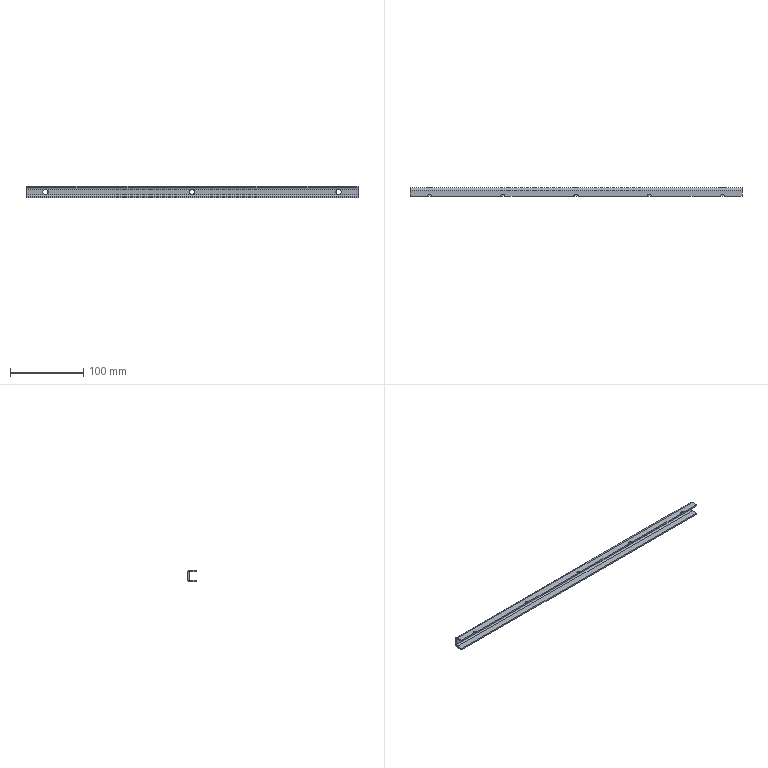Part | NX | features solid 2 | 1 solid | 35 faces | box 453 x 12 x 16 mm | volume 29904 mm3 | cylinder 20 | plane 15 | commonest cylinder face diameters 6 x10 7.1 x6 4 x2 8 x2
STEP:
#1=CARTESIAN_POINT('',(1406.5,-1575.5,344.5));
#2=VERTEX_POINT('',#1);
#3=CARTESIAN_POINT('',(1406.5,-1575.5,346.5));
#4=VERTEX_POINT('',#3);
#5=CARTESIAN_POINT('',(1406.5,-1575.5,346.5));
#6=DIRECTION('',(0.,0.,1.));
#7=VECTOR('',#6,1000.);
#8=LINE('',#5,#7);
#9=EDGE_CURVE('',#2,#4,#8,.T.);
#10=ORIENTED_EDGE('',*,*,#9,.F.);
#11=CARTESIAN_POINT('',(1409.5,-1578.5,344.5));
#12=VERTEX_POINT('',#11);
#13=CARTESIAN_POINT('',(1406.5,-1578.5,344.5));
#14=DIRECTION('',(0.,0.,-1.));
#15=DIRECTION('',(0.,1.,0.));
#16=AXIS2_PLACEMENT_3D('',#13,#14,#15);
#17=CIRCLE('',#16,3.);
#18=EDGE_CURVE('',#2,#12,#17,.T.);
#19=ORIENTED_EDGE('',*,*,#18,.T.);
#20=CARTESIAN_POINT('',(1409.5,-1578.5,346.5));
#21=VERTEX_POINT('',#20);
#22=CARTESIAN_POINT('',(1409.5,-1578.5,346.5));
#23=DIRECTION('',(0.,0.,1.));
#24=VECTOR('',#23,1000.);
#25=LINE('',#22,#24);
#26=EDGE_CURVE('',#12,#21,#25,.T.);
#27=ORIENTED_EDGE('',*,*,#26,.T.);
#28=CARTESIAN_POINT('',(1406.5,-1578.5,346.5));
#29=DIRECTION('',(0.,0.,-1.));
#30=DIRECTION('',(0.,1.,0.));
#31=AXIS2_PLACEMENT_3D('',#28,#29,#30);
#32=CIRCLE('',#31,3.);
#33=EDGE_CURVE('',#4,#21,#32,.T.);
#34=ORIENTED_EDGE('',*,*,#33,.F.);
#35=EDGE_LOOP('',(#10,#19,#27,#34));
#36=FACE_BOUND('',#35,.T.);
#37=CARTESIAN_POINT('',(1406.5,-1578.5,346.5));
#38=DIRECTION('',(0.,0.,1.));
#39=DIRECTION('',(0.,1.,0.));
#40=AXIS2_PLACEMENT_3D('',#37,#38,#39);
#41=CYLINDRICAL_SURFACE('',#40,3.);
#42=ADVANCED_FACE('',(#36),#41,.F.);
#43=CARTESIAN_POINT('',(1506.5,-1575.5,344.5));
#44=VERTEX_POINT('',#43);
#45=CARTESIAN_POINT('',(1506.5,-1575.5,346.5));
#46=VERTEX_POINT('',#45);
#47=CARTESIAN_POINT('',(1506.5,-1575.5,346.5));
#48=DIRECTION('',(0.,0.,1.));
#49=VECTOR('',#48,1000.);
#50=LINE('',#47,#49);
#51=EDGE_CURVE('',#44,#46,#50,.T.);
#52=ORIENTED_EDGE('',*,*,#51,.F.);
#53=CARTESIAN_POINT('',(1509.5,-1578.5,344.5));
#54=VERTEX_POINT('',#53);
#55=CARTESIAN_POINT('',(1506.5,-1578.5,344.5));
#56=DIRECTION('',(0.,0.,-1.));
#57=DIRECTION('',(0.,1.,0.));
#58=AXIS2_PLACEMENT_3D('',#55,#56,#57);
#59=CIRCLE('',#58,3.);
#60=EDGE_CURVE('',#44,#54,#59,.T.);
#61=ORIENTED_EDGE('',*,*,#60,.T.);
#62=CARTESIAN_POINT('',(1509.5,-1578.5,346.5));
#63=VERTEX_POINT('',#62);
#64=CARTESIAN_POINT('',(1509.5,-1578.5,346.5));
#65=DIRECTION('',(0.,0.,1.));
#66=VECTOR('',#65,1000.);
#67=LINE('',#64,#66);
#68=EDGE_CURVE('',#54,#63,#67,.T.);
#69=ORIENTED_EDGE('',*,*,#68,.T.);
#70=CARTESIAN_POINT('',(1506.5,-1578.5,346.5));
#71=DIRECTION('',(0.,0.,-1.));
#72=DIRECTION('',(0.,1.,0.));
#73=AXIS2_PLACEMENT_3D('',#70,#71,#72);
#74=CIRCLE('',#73,3.);
#75=EDGE_CURVE('',#46,#63,#74,.T.);
#76=ORIENTED_EDGE('',*,*,#75,.F.);
#77=EDGE_LOOP('',(#52,#61,#69,#76));
#78=FACE_BOUND('',#77,.T.);
#79=CARTESIAN_POINT('',(1506.5,-1578.5,346.5));
#80=DIRECTION('',(0.,0.,1.));
#81=DIRECTION('',(0.,1.,0.));
#82=AXIS2_PLACEMENT_3D('',#79,#80,#81);
#83=CYLINDRICAL_SURFACE('',#82,3.);
#84=ADVANCED_FACE('',(#78),#83,.F.);
#85=CARTESIAN_POINT('',(1806.5,-1575.5,344.5));
#86=VERTEX_POINT('',#85);
#87=CARTESIAN_POINT('',(1806.5,-1575.5,346.5));
#88=VERTEX_POINT('',#87);
#89=CARTESIAN_POINT('',(1806.5,-1575.5,346.5));
#90=DIRECTION('',(0.,0.,1.));
#91=VECTOR('',#90,1000.);
#92=LINE('',#89,#91);
#93=EDGE_CURVE('',#86,#88,#92,.T.);
#94=ORIENTED_EDGE('',*,*,#93,.F.);
#95=CARTESIAN_POINT('',(1809.5,-1578.5,344.5));
#96=VERTEX_POINT('',#95);
#97=CARTESIAN_POINT('',(1806.5,-1578.5,344.5));
#98=DIRECTION('',(0.,0.,-1.));
#99=DIRECTION('',(0.,1.,0.));
#100=AXIS2_PLACEMENT_3D('',#97,#98,#99);
#101=CIRCLE('',#100,3.);
#102=EDGE_CURVE('',#86,#96,#101,.T.);
#103=ORIENTED_EDGE('',*,*,#102,.T.);
#104=CARTESIAN_POINT('',(1809.5,-1578.5,346.5));
#105=VERTEX_POINT('',#104);
#106=CARTESIAN_POINT('',(1809.5,-1578.5,346.5));
#107=DIRECTION('',(0.,0.,1.));
#108=VECTOR('',#107,1000.);
#109=LINE('',#106,#108);
#110=EDGE_CURVE('',#96,#105,#109,.T.);
#111=ORIENTED_EDGE('',*,*,#110,.T.);
#112=CARTESIAN_POINT('',(1806.5,-1578.5,346.5));
#113=DIRECTION('',(0.,0.,-1.));
#114=DIRECTION('',(0.,1.,0.));
#115=AXIS2_PLACEMENT_3D('',#112,#113,#114);
#116=CIRCLE('',#115,3.);
#117=EDGE_CURVE('',#88,#105,#116,.T.);
#118=ORIENTED_EDGE('',*,*,#117,.F.);
#119=EDGE_LOOP('',(#94,#103,#111,#118));
#120=FACE_BOUND('',#119,.T.);
#121=CARTESIAN_POINT('',(1806.5,-1578.5,346.5));
#122=DIRECTION('',(0.,0.,1.));
#123=DIRECTION('',(0.,1.,0.));
#124=AXIS2_PLACEMENT_3D('',#121,#122,#123);
#125=CYLINDRICAL_SURFACE('',#124,3.);
#126=ADVANCED_FACE('',(#120),#125,.F.);
#127=CARTESIAN_POINT('',(1706.5,-1575.5,344.5));
#128=VERTEX_POINT('',#127);
#129=CARTESIAN_POINT('',(1706.5,-1575.5,346.5));
#130=VERTEX_POINT('',#129);
#131=CARTESIAN_POINT('',(1706.5,-1575.5,346.5));
#132=DIRECTION('',(0.,0.,1.));
#133=VECTOR('',#132,1000.);
#134=LINE('',#131,#133);
#135=EDGE_CURVE('',#128,#130,#134,.T.);
#136=ORIENTED_EDGE('',*,*,#135,.F.);
#137=CARTESIAN_POINT('',(1709.5,-1578.5,344.5));
#138=VERTEX_POINT('',#137);
#139=CARTESIAN_POINT('',(1706.5,-1578.5,344.5));
#140=DIRECTION('',(0.,0.,-1.));
#141=DIRECTION('',(0.,1.,0.));
#142=AXIS2_PLACEMENT_3D('',#139,#140,#141);
#143=CIRCLE('',#142,3.);
#144=EDGE_CURVE('',#128,#138,#143,.T.);
#145=ORIENTED_EDGE('',*,*,#144,.T.);
#146=CARTESIAN_POINT('',(1709.5,-1578.5,346.5));
#147=VERTEX_POINT('',#146);
#148=CARTESIAN_POINT('',(1709.5,-1578.5,346.5));
#149=DIRECTION('',(0.,0.,1.));
#150=VECTOR('',#149,1000.);
#151=LINE('',#148,#150);
#152=EDGE_CURVE('',#138,#147,#151,.T.);
#153=ORIENTED_EDGE('',*,*,#152,.T.);
#154=CARTESIAN_POINT('',(1706.5,-1578.5,346.5));
#155=DIRECTION('',(0.,0.,-1.));
#156=DIRECTION('',(0.,1.,0.));
#157=AXIS2_PLACEMENT_3D('',#154,#155,#156);
#158=CIRCLE('',#157,3.);
#159=EDGE_CURVE('',#130,#147,#158,.T.);
#160=ORIENTED_EDGE('',*,*,#159,.F.);
#161=EDGE_LOOP('',(#136,#145,#153,#160));
#162=FACE_BOUND('',#161,.T.);
#163=CARTESIAN_POINT('',(1706.5,-1578.5,346.5));
#164=DIRECTION('',(0.,0.,1.));
#165=DIRECTION('',(0.,1.,0.));
#166=AXIS2_PLACEMENT_3D('',#163,#164,#165);
#167=CYLINDRICAL_SURFACE('',#166,3.);
#168=ADVANCED_FACE('',(#162),#167,.F.);
#169=CARTESIAN_POINT('',(1606.5,-1575.5,344.5));
#170=VERTEX_POINT('',#169);
#171=CARTESIAN_POINT('',(1606.5,-1575.5,346.5));
#172=VERTEX_POINT('',#171);
#173=CARTESIAN_POINT('',(1606.5,-1575.5,346.5));
#174=DIRECTION('',(0.,0.,1.));
#175=VECTOR('',#174,1000.);
#176=LINE('',#173,#175);
#177=EDGE_CURVE('',#170,#172,#176,.T.);
#178=ORIENTED_EDGE('',*,*,#177,.F.);
#179=CARTESIAN_POINT('',(1609.5,-1578.5,344.5));
#180=VERTEX_POINT('',#179);
#181=CARTESIAN_POINT('',(1606.5,-1578.5,344.5));
#182=DIRECTION('',(0.,0.,-1.));
#183=DIRECTION('',(0.,1.,0.));
#184=AXIS2_PLACEMENT_3D('',#181,#182,#183);
#185=CIRCLE('',#184,3.);
#186=EDGE_CURVE('',#170,#180,#185,.T.);
#187=ORIENTED_EDGE('',*,*,#186,.T.);
#188=CARTESIAN_POINT('',(1609.5,-1578.5,346.5));
#189=VERTEX_POINT('',#188);
#190=CARTESIAN_POINT('',(1609.5,-1578.5,346.5));
#191=DIRECTION('',(0.,0.,1.));
#192=VECTOR('',#191,1000.);
#193=LINE('',#190,#192);
#194=EDGE_CURVE('',#180,#189,#193,.T.);
#195=ORIENTED_EDGE('',*,*,#194,.T.);
#196=CARTESIAN_POINT('',(1606.5,-1578.5,346.5));
#197=DIRECTION('',(0.,0.,-1.));
#198=DIRECTION('',(0.,1.,0.));
#199=AXIS2_PLACEMENT_3D('',#196,#197,#198);
#200=CIRCLE('',#199,3.);
#201=EDGE_CURVE('',#172,#189,#200,.T.);
#202=ORIENTED_EDGE('',*,*,#201,.F.);
#203=EDGE_LOOP('',(#178,#187,#195,#202));
#204=FACE_BOUND('',#203,.T.);
#205=CARTESIAN_POINT('',(1606.5,-1578.5,346.5));
#206=DIRECTION('',(0.,0.,1.));
#207=DIRECTION('',(0.,1.,0.));
#208=AXIS2_PLACEMENT_3D('',#205,#206,#207);
#209=CYLINDRICAL_SURFACE('',#208,3.);
#210=ADVANCED_FACE('',(#204),#209,.F.);
#211=CARTESIAN_POINT('',(1380.,-1568.5,342.5));
#212=VERTEX_POINT('',#211);
#213=CARTESIAN_POINT('',(1833.,-1568.5,342.5));
#214=VERTEX_POINT('',#213);
#215=CARTESIAN_POINT('',(1380.,-1568.5,342.5));
#216=DIRECTION('',(1.,0.,0.));
#217=VECTOR('',#216,1000.);
#218=LINE('',#215,#217);
#219=EDGE_CURVE('',#212,#214,#218,.T.);
#220=ORIENTED_EDGE('',*,*,#219,.T.);
#221=CARTESIAN_POINT('',(1833.,-1570.5,344.5));
#222=VERTEX_POINT('',#221);
#223=CARTESIAN_POINT('',(1833.,-1570.5,342.5));
#224=DIRECTION('',(-1.,0.,0.));
#225=DIRECTION('',(0.,0.,1.));
#226=AXIS2_PLACEMENT_3D('',#223,#224,#225);
#227=CIRCLE('',#226,2.);
#228=EDGE_CURVE('',#222,#214,#227,.T.);
#229=ORIENTED_EDGE('',*,*,#228,.F.);
#230=CARTESIAN_POINT('',(1380.,-1570.5,344.5));
#231=VERTEX_POINT('',#230);
#232=CARTESIAN_POINT('',(1833.,-1570.5,344.5));
#233=DIRECTION('',(-1.,0.,0.));
#234=VECTOR('',#233,1000.);
#235=LINE('',#232,#234);
#236=EDGE_CURVE('',#222,#231,#235,.T.);
#237=ORIENTED_EDGE('',*,*,#236,.T.);
#238=CARTESIAN_POINT('',(1380.,-1570.5,342.5));
#239=DIRECTION('',(1.,0.,0.));
#240=DIRECTION('',(0.,0.,1.));
#241=AXIS2_PLACEMENT_3D('',#238,#239,#240);
#242=CIRCLE('',#241,2.);
#243=EDGE_CURVE('',#212,#231,#242,.T.);
#244=ORIENTED_EDGE('',*,*,#243,.F.);
#245=EDGE_LOOP('',(#220,#229,#237,#244));
#246=FACE_BOUND('',#245,.T.);
#247=CARTESIAN_POINT('',(1380.,-1570.5,342.5));
#248=DIRECTION('',(1.,0.,0.));
#249=DIRECTION('',(0.,-1.,0.));
#250=AXIS2_PLACEMENT_3D('',#247,#248,#249);
#251=CYLINDRICAL_SURFACE('',#250,2.);
#252=ADVANCED_FACE('',(#246),#251,.F.);
#253=CARTESIAN_POINT('',(1380.,-1566.5,342.5));
#254=VERTEX_POINT('',#253);
#255=CARTESIAN_POINT('',(1833.,-1566.5,342.5));
#256=VERTEX_POINT('',#255);
#257=CARTESIAN_POINT('',(1380.,-1566.5,342.5));
#258=DIRECTION('',(1.,0.,0.));
#259=VECTOR('',#258,1000.);
#260=LINE('',#257,#259);
#261=EDGE_CURVE('',#254,#256,#260,.T.);
#262=ORIENTED_EDGE('',*,*,#261,.F.);
#263=CARTESIAN_POINT('',(1380.,-1570.5,346.5));
#264=VERTEX_POINT('',#263);
#265=CARTESIAN_POINT('',(1380.,-1570.5,342.5));
#266=DIRECTION('',(1.,0.,0.));
#267=DIRECTION('',(0.,-1.,0.));
#268=AXIS2_PLACEMENT_3D('',#265,#266,#267);
#269=CIRCLE('',#268,4.);
#270=EDGE_CURVE('',#254,#264,#269,.T.);
#271=ORIENTED_EDGE('',*,*,#270,.T.);
#272=CARTESIAN_POINT('',(1833.,-1570.5,346.5));
#273=VERTEX_POINT('',#272);
#274=CARTESIAN_POINT('',(1833.,-1570.5,346.5));
#275=DIRECTION('',(-1.,0.,0.));
#276=VECTOR('',#275,1000.);
#277=LINE('',#274,#276);
#278=EDGE_CURVE('',#273,#264,#277,.T.);
#279=ORIENTED_EDGE('',*,*,#278,.F.);
#280=CARTESIAN_POINT('',(1833.,-1570.5,342.5));
#281=DIRECTION('',(-1.,0.,0.));
#282=DIRECTION('',(0.,-1.,0.));
#283=AXIS2_PLACEMENT_3D('',#280,#281,#282);
#284=CIRCLE('',#283,4.);
#285=EDGE_CURVE('',#273,#256,#284,.T.);
#286=ORIENTED_EDGE('',*,*,#285,.T.);
#287=EDGE_LOOP('',(#262,#271,#279,#286));
#288=FACE_BOUND('',#287,.T.);
#289=CARTESIAN_POINT('',(1380.,-1570.5,342.5));
#290=DIRECTION('',(1.,0.,0.));
#291=DIRECTION('',(0.,-1.,0.));
#292=AXIS2_PLACEMENT_3D('',#289,#290,#291);
#293=CYLINDRICAL_SURFACE('',#292,4.);
#294=ADVANCED_FACE('',(#288),#293,.T.);
#295=CARTESIAN_POINT('',(1833.,-1578.5,346.5));
#296=VERTEX_POINT('',#295);
#297=CARTESIAN_POINT('',(1380.,-1578.5,346.5));
#298=DIRECTION('',(1.,0.,0.));
#299=VECTOR('',#298,1000.);
#300=LINE('',#297,#299);
#301=EDGE_CURVE('',#105,#296,#300,.T.);
#302=ORIENTED_EDGE('',*,*,#301,.F.);
#303=ORIENTED_EDGE('',*,*,#110,.F.);
#304=CARTESIAN_POINT('',(1833.,-1578.5,344.5));
#305=VERTEX_POINT('',#304);
#306=CARTESIAN_POINT('',(1380.,-1578.5,344.5));
#307=DIRECTION('',(1.,0.,0.));
#308=VECTOR('',#307,1000.);
#309=LINE('',#306,#308);
#310=EDGE_CURVE('',#96,#305,#309,.T.);
#311=ORIENTED_EDGE('',*,*,#310,.T.);
#312=CARTESIAN_POINT('',(1833.,-1578.5,346.5));
#313=DIRECTION('',(0.,0.,-1.));
#314=VECTOR('',#313,1000.);
#315=LINE('',#312,#314);
#316=EDGE_CURVE('',#296,#305,#315,.T.);
#317=ORIENTED_EDGE('',*,*,#316,.F.);
#318=EDGE_LOOP('',(#302,#303,#311,#317));
#319=FACE_BOUND('',#318,.T.);
#320=CARTESIAN_POINT('',(1380.,-1578.5,346.5));
#321=DIRECTION('',(0.,1.,0.));
#322=DIRECTION('',(0.,0.,-1.));
#323=AXIS2_PLACEMENT_3D('',#320,#321,#322);
#324=PLANE('',#323);
#325=ADVANCED_FACE('',(#319),#324,.F.);
#326=CARTESIAN_POINT('',(1503.5,-1578.5,344.5));
#327=VERTEX_POINT('',#326);
#328=CARTESIAN_POINT('',(1380.,-1578.5,344.5));
#329=DIRECTION('',(1.,0.,0.));
#330=VECTOR('',#329,1000.);
#331=LINE('',#328,#330);
#332=EDGE_CURVE('',#12,#327,#331,.T.);
#333=ORIENTED_EDGE('',*,*,#332,.F.);
#334=ORIENTED_EDGE('',*,*,#18,.F.);
#335=CARTESIAN_POINT('',(1403.5,-1578.5,344.5));
#336=VERTEX_POINT('',#335);
#337=CARTESIAN_POINT('',(1406.5,-1578.5,344.5));
#338=DIRECTION('',(0.,0.,-1.));
#339=DIRECTION('',(0.,1.,0.));
#340=AXIS2_PLACEMENT_3D('',#337,#338,#339);
#341=CIRCLE('',#340,3.);
#342=EDGE_CURVE('',#336,#2,#341,.T.);
#343=ORIENTED_EDGE('',*,*,#342,.F.);
#344=CARTESIAN_POINT('',(1380.,-1578.5,344.5));
#345=VERTEX_POINT('',#344);
#346=CARTESIAN_POINT('',(1380.,-1578.5,344.5));
#347=DIRECTION('',(1.,0.,0.));
#348=VECTOR('',#347,1000.);
#349=LINE('',#346,#348);
#350=EDGE_CURVE('',#345,#336,#349,.T.);
#351=ORIENTED_EDGE('',*,*,#350,.F.);
#352=CARTESIAN_POINT('',(1380.,-1568.144,344.5));
#353=DIRECTION('',(0.,-1.,0.));
#354=VECTOR('',#353,1000.);
#355=LINE('',#352,#354);
#356=EDGE_CURVE('',#231,#345,#355,.T.);
#357=ORIENTED_EDGE('',*,*,#356,.F.);
#358=ORIENTED_EDGE('',*,*,#236,.F.);
#359=CARTESIAN_POINT('',(1833.,-1568.144,344.5));
#360=DIRECTION('',(0.,1.,0.));
#361=VECTOR('',#360,1000.);
#362=LINE('',#359,#361);
#363=EDGE_CURVE('',#305,#222,#362,.T.);
#364=ORIENTED_EDGE('',*,*,#363,.F.);
#365=ORIENTED_EDGE('',*,*,#310,.F.);
#366=ORIENTED_EDGE('',*,*,#102,.F.);
#367=CARTESIAN_POINT('',(1803.5,-1578.5,344.5));
#368=VERTEX_POINT('',#367);
#369=CARTESIAN_POINT('',(1806.5,-1578.5,344.5));
#370=DIRECTION('',(0.,0.,-1.));
#371=DIRECTION('',(0.,1.,0.));
#372=AXIS2_PLACEMENT_3D('',#369,#370,#371);
#373=CIRCLE('',#372,3.);
#374=EDGE_CURVE('',#368,#86,#373,.T.);
#375=ORIENTED_EDGE('',*,*,#374,.F.);
#376=CARTESIAN_POINT('',(1380.,-1578.5,344.5));
#377=DIRECTION('',(1.,0.,0.));
#378=VECTOR('',#377,1000.);
#379=LINE('',#376,#378);
#380=EDGE_CURVE('',#138,#368,#379,.T.);
#381=ORIENTED_EDGE('',*,*,#380,.F.);
#382=ORIENTED_EDGE('',*,*,#144,.F.);
#383=CARTESIAN_POINT('',(1703.5,-1578.5,344.5));
#384=VERTEX_POINT('',#383);
#385=CARTESIAN_POINT('',(1706.5,-1578.5,344.5));
#386=DIRECTION('',(0.,0.,-1.));
#387=DIRECTION('',(0.,1.,0.));
#388=AXIS2_PLACEMENT_3D('',#385,#386,#387);
#389=CIRCLE('',#388,3.);
#390=EDGE_CURVE('',#384,#128,#389,.T.);
#391=ORIENTED_EDGE('',*,*,#390,.F.);
#392=CARTESIAN_POINT('',(1380.,-1578.5,344.5));
#393=DIRECTION('',(1.,0.,0.));
#394=VECTOR('',#393,1000.);
#395=LINE('',#392,#394);
#396=EDGE_CURVE('',#180,#384,#395,.T.);
#397=ORIENTED_EDGE('',*,*,#396,.F.);
#398=ORIENTED_EDGE('',*,*,#186,.F.);
#399=CARTESIAN_POINT('',(1603.5,-1578.5,344.5));
#400=VERTEX_POINT('',#399);
#401=CARTESIAN_POINT('',(1606.5,-1578.5,344.5));
#402=DIRECTION('',(0.,0.,-1.));
#403=DIRECTION('',(0.,1.,0.));
#404=AXIS2_PLACEMENT_3D('',#401,#402,#403);
#405=CIRCLE('',#404,3.);
#406=EDGE_CURVE('',#400,#170,#405,.T.);
#407=ORIENTED_EDGE('',*,*,#406,.F.);
#408=CARTESIAN_POINT('',(1380.,-1578.5,344.5));
#409=DIRECTION('',(1.,0.,0.));
#410=VECTOR('',#409,1000.);
#411=LINE('',#408,#410);
#412=EDGE_CURVE('',#54,#400,#411,.T.);
#413=ORIENTED_EDGE('',*,*,#412,.F.);
#414=ORIENTED_EDGE('',*,*,#60,.F.);
#415=CARTESIAN_POINT('',(1506.5,-1578.5,344.5));
#416=DIRECTION('',(0.,0.,-1.));
#417=DIRECTION('',(0.,1.,0.));
#418=AXIS2_PLACEMENT_3D('',#415,#416,#417);
#419=CIRCLE('',#418,3.);
#420=EDGE_CURVE('',#327,#44,#419,.T.);
#421=ORIENTED_EDGE('',*,*,#420,.F.);
#422=EDGE_LOOP('',(#333,#334,#343,#351,#357,#358,#364,#365,#366,#375,#381,#382,#391,#397,#398,#407,#413,#414,#421));
#423=FACE_BOUND('',#422,.T.);
#424=CARTESIAN_POINT('',(1606.5,-1566.5,344.5));
#425=DIRECTION('',(0.,0.,1.));
#426=DIRECTION('',(1.,0.,0.));
#427=AXIS2_PLACEMENT_3D('',#424,#425,#426);
#428=PLANE('',#427);
#429=ADVANCED_FACE('',(#423),#428,.F.);
#430=CARTESIAN_POINT('',(1403.5,-1578.5,346.5));
#431=VERTEX_POINT('',#430);
#432=CARTESIAN_POINT('',(1406.5,-1578.5,346.5));
#433=DIRECTION('',(0.,0.,-1.));
#434=DIRECTION('',(0.,1.,0.));
#435=AXIS2_PLACEMENT_3D('',#432,#433,#434);
#436=CIRCLE('',#435,3.);
#437=EDGE_CURVE('',#431,#4,#436,.T.);
#438=ORIENTED_EDGE('',*,*,#437,.T.);
#439=ORIENTED_EDGE('',*,*,#33,.T.);
#440=CARTESIAN_POINT('',(1503.5,-1578.5,346.5));
#441=VERTEX_POINT('',#440);
#442=CARTESIAN_POINT('',(1380.,-1578.5,346.5));
#443=DIRECTION('',(1.,0.,0.));
#444=VECTOR('',#443,1000.);
#445=LINE('',#442,#444);
#446=EDGE_CURVE('',#21,#441,#445,.T.);
#447=ORIENTED_EDGE('',*,*,#446,.T.);
#448=CARTESIAN_POINT('',(1506.5,-1578.5,346.5));
#449=DIRECTION('',(0.,0.,-1.));
#450=DIRECTION('',(0.,1.,0.));
#451=AXIS2_PLACEMENT_3D('',#448,#449,#450);
#452=CIRCLE('',#451,3.);
#453=EDGE_CURVE('',#441,#46,#452,.T.);
#454=ORIENTED_EDGE('',*,*,#453,.T.);
#455=ORIENTED_EDGE('',*,*,#75,.T.);
#456=CARTESIAN_POINT('',(1603.5,-1578.5,346.5));
#457=VERTEX_POINT('',#456);
#458=CARTESIAN_POINT('',(1380.,-1578.5,346.5));
#459=DIRECTION('',(1.,0.,0.));
#460=VECTOR('',#459,1000.);
#461=LINE('',#458,#460);
#462=EDGE_CURVE('',#63,#457,#461,.T.);
#463=ORIENTED_EDGE('',*,*,#462,.T.);
#464=CARTESIAN_POINT('',(1606.5,-1578.5,346.5));
#465=DIRECTION('',(0.,0.,-1.));
#466=DIRECTION('',(0.,1.,0.));
#467=AXIS2_PLACEMENT_3D('',#464,#465,#466);
#468=CIRCLE('',#467,3.);
#469=EDGE_CURVE('',#457,#172,#468,.T.);
#470=ORIENTED_EDGE('',*,*,#469,.T.);
#471=ORIENTED_EDGE('',*,*,#201,.T.);
#472=CARTESIAN_POINT('',(1703.5,-1578.5,346.5));
#473=VERTEX_POINT('',#472);
#474=CARTESIAN_POINT('',(1380.,-1578.5,346.5));
#475=DIRECTION('',(1.,0.,0.));
#476=VECTOR('',#475,1000.);
#477=LINE('',#474,#476);
#478=EDGE_CURVE('',#189,#473,#477,.T.);
#479=ORIENTED_EDGE('',*,*,#478,.T.);
#480=CARTESIAN_POINT('',(1706.5,-1578.5,346.5));
#481=DIRECTION('',(0.,0.,-1.));
#482=DIRECTION('',(0.,1.,0.));
#483=AXIS2_PLACEMENT_3D('',#480,#481,#482);
#484=CIRCLE('',#483,3.);
#485=EDGE_CURVE('',#473,#130,#484,.T.);
#486=ORIENTED_EDGE('',*,*,#485,.T.);
#487=ORIENTED_EDGE('',*,*,#159,.T.);
#488=CARTESIAN_POINT('',(1803.5,-1578.5,346.5));
#489=VERTEX_POINT('',#488);
#490=CARTESIAN_POINT('',(1380.,-1578.5,346.5));
#491=DIRECTION('',(1.,0.,0.));
#492=VECTOR('',#491,1000.);
#493=LINE('',#490,#492);
#494=EDGE_CURVE('',#147,#489,#493,.T.);
#495=ORIENTED_EDGE('',*,*,#494,.T.);
#496=CARTESIAN_POINT('',(1806.5,-1578.5,346.5));
#497=DIRECTION('',(0.,0.,-1.));
#498=DIRECTION('',(0.,1.,0.));
#499=AXIS2_PLACEMENT_3D('',#496,#497,#498);
#500=CIRCLE('',#499,3.);
#501=EDGE_CURVE('',#489,#88,#500,.T.);
#502=ORIENTED_EDGE('',*,*,#501,.T.);
#503=ORIENTED_EDGE('',*,*,#117,.T.);
#504=ORIENTED_EDGE('',*,*,#301,.T.);
#505=CARTESIAN_POINT('',(1833.,-1568.144,346.5));
#506=DIRECTION('',(0.,1.,0.));
#507=VECTOR('',#506,1000.);
#508=LINE('',#505,#507);
#509=EDGE_CURVE('',#296,#273,#508,.T.);
#510=ORIENTED_EDGE('',*,*,#509,.T.);
#511=ORIENTED_EDGE('',*,*,#278,.T.);
#512=CARTESIAN_POINT('',(1380.,-1578.5,346.5));
#513=VERTEX_POINT('',#512);
#514=CARTESIAN_POINT('',(1380.,-1568.144,346.5));
#515=DIRECTION('',(0.,-1.,0.));
#516=VECTOR('',#515,1000.);
#517=LINE('',#514,#516);
#518=EDGE_CURVE('',#264,#513,#517,.T.);
#519=ORIENTED_EDGE('',*,*,#518,.T.);
#520=CARTESIAN_POINT('',(1380.,-1578.5,346.5));
#521=DIRECTION('',(1.,0.,0.));
#522=VECTOR('',#521,1000.);
#523=LINE('',#520,#522);
#524=EDGE_CURVE('',#513,#431,#523,.T.);
#525=ORIENTED_EDGE('',*,*,#524,.T.);
#526=EDGE_LOOP('',(#438,#439,#447,#454,#455,#463,#470,#471,#479,#486,#487,#495,#502,#503,#504,#510,#511,#519,#525));
#527=FACE_BOUND('',#526,.T.);
#528=CARTESIAN_POINT('',(1606.5,-1566.5,346.5));
#529=DIRECTION('',(0.,0.,1.));
#530=DIRECTION('',(1.,0.,0.));
#531=AXIS2_PLACEMENT_3D('',#528,#529,#530);
#532=PLANE('',#531);
#533=ADVANCED_FACE('',(#527),#532,.T.);
#534=CARTESIAN_POINT('',(1833.,-1568.5,334.5));
#535=VERTEX_POINT('',#534);
#536=CARTESIAN_POINT('',(1380.,-1568.5,334.5));
#537=VERTEX_POINT('',#536);
#538=CARTESIAN_POINT('',(1833.,-1568.5,334.5));
#539=DIRECTION('',(-1.,0.,0.));
#540=VECTOR('',#539,1000.);
#541=LINE('',#538,#540);
#542=EDGE_CURVE('',#535,#537,#541,.T.);
#543=ORIENTED_EDGE('',*,*,#542,.T.);
#544=CARTESIAN_POINT('',(1380.,-1570.5,332.5));
#545=VERTEX_POINT('',#544);
#546=CARTESIAN_POINT('',(1380.,-1570.5,334.5));
#547=DIRECTION('',(1.,0.,0.));
#548=DIRECTION('',(0.,0.,-1.));
#549=AXIS2_PLACEMENT_3D('',#546,#547,#548);
#550=CIRCLE('',#549,2.);
#551=EDGE_CURVE('',#545,#537,#550,.T.);
#552=ORIENTED_EDGE('',*,*,#551,.F.);
#553=CARTESIAN_POINT('',(1833.,-1570.5,332.5));
#554=VERTEX_POINT('',#553);
#555=CARTESIAN_POINT('',(1380.,-1570.5,332.5));
#556=DIRECTION('',(1.,0.,0.));
#557=VECTOR('',#556,1000.);
#558=LINE('',#555,#557);
#559=EDGE_CURVE('',#545,#554,#558,.T.);
#560=ORIENTED_EDGE('',*,*,#559,.T.);
#561=CARTESIAN_POINT('',(1833.,-1570.5,334.5));
#562=DIRECTION('',(-1.,0.,0.));
#563=DIRECTION('',(0.,0.,-1.));
#564=AXIS2_PLACEMENT_3D('',#561,#562,#563);
#565=CIRCLE('',#564,2.);
#566=EDGE_CURVE('',#535,#554,#565,.T.);
#567=ORIENTED_EDGE('',*,*,#566,.F.);
#568=EDGE_LOOP('',(#543,#552,#560,#567));
#569=FACE_BOUND('',#568,.T.);
#570=CARTESIAN_POINT('',(1833.,-1570.5,334.5));
#571=DIRECTION('',(-1.,0.,0.));
#572=DIRECTION('',(0.,-1.,0.));
#573=AXIS2_PLACEMENT_3D('',#570,#571,#572);
#574=CYLINDRICAL_SURFACE('',#573,2.);
#575=ADVANCED_FACE('',(#569),#574,.F.);
#576=CARTESIAN_POINT('',(1833.,-1566.5,334.5));
#577=VERTEX_POINT('',#576);
#578=CARTESIAN_POINT('',(1380.,-1566.5,334.5));
#579=VERTEX_POINT('',#578);
#580=CARTESIAN_POINT('',(1833.,-1566.5,334.5));
#581=DIRECTION('',(-1.,0.,0.));
#582=VECTOR('',#581,1000.);
#583=LINE('',#580,#582);
#584=EDGE_CURVE('',#577,#579,#583,.T.);
#585=ORIENTED_EDGE('',*,*,#584,.F.);
#586=CARTESIAN_POINT('',(1833.,-1570.5,330.5));
#587=VERTEX_POINT('',#586);
#588=CARTESIAN_POINT('',(1833.,-1570.5,334.5));
#589=DIRECTION('',(-1.,0.,0.));
#590=DIRECTION('',(0.,-1.,0.));
#591=AXIS2_PLACEMENT_3D('',#588,#589,#590);
#592=CIRCLE('',#591,4.);
#593=EDGE_CURVE('',#577,#587,#592,.T.);
#594=ORIENTED_EDGE('',*,*,#593,.T.);
#595=CARTESIAN_POINT('',(1380.,-1570.5,330.5));
#596=VERTEX_POINT('',#595);
#597=CARTESIAN_POINT('',(1380.,-1570.5,330.5));
#598=DIRECTION('',(1.,0.,0.));
#599=VECTOR('',#598,1000.);
#600=LINE('',#597,#599);
#601=EDGE_CURVE('',#596,#587,#600,.T.);
#602=ORIENTED_EDGE('',*,*,#601,.F.);
#603=CARTESIAN_POINT('',(1380.,-1570.5,334.5));
#604=DIRECTION('',(1.,0.,0.));
#605=DIRECTION('',(0.,-1.,0.));
#606=AXIS2_PLACEMENT_3D('',#603,#604,#605);
#607=CIRCLE('',#606,4.);
#608=EDGE_CURVE('',#596,#579,#607,.T.);
#609=ORIENTED_EDGE('',*,*,#608,.T.);
#610=EDGE_LOOP('',(#585,#594,#602,#609));
#611=FACE_BOUND('',#610,.T.);
#612=CARTESIAN_POINT('',(1833.,-1570.5,334.5));
#613=DIRECTION('',(-1.,0.,0.));
#614=DIRECTION('',(0.,-1.,0.));
#615=AXIS2_PLACEMENT_3D('',#612,#613,#614);
#616=CYLINDRICAL_SURFACE('',#615,4.);
#617=ADVANCED_FACE('',(#611),#616,.T.);
#618=CARTESIAN_POINT('',(1833.,-1578.5,332.5));
#619=VERTEX_POINT('',#618);
#620=CARTESIAN_POINT('',(1380.,-1578.5,332.5));
#621=VERTEX_POINT('',#620);
#622=CARTESIAN_POINT('',(1833.,-1578.5,332.5));
#623=DIRECTION('',(-1.,0.,0.));
#624=VECTOR('',#623,1000.);
#625=LINE('',#622,#624);
#626=EDGE_CURVE('',#619,#621,#625,.T.);
#627=ORIENTED_EDGE('',*,*,#626,.T.);
#628=CARTESIAN_POINT('',(1380.,-1578.5,330.5));
#629=VERTEX_POINT('',#628);
#630=CARTESIAN_POINT('',(1380.,-1578.5,330.5));
#631=DIRECTION('',(0.,0.,1.));
#632=VECTOR('',#631,1000.);
#633=LINE('',#630,#632);
#634=EDGE_CURVE('',#629,#621,#633,.T.);
#635=ORIENTED_EDGE('',*,*,#634,.F.);
#636=CARTESIAN_POINT('',(1833.,-1578.5,330.5));
#637=VERTEX_POINT('',#636);
#638=CARTESIAN_POINT('',(1833.,-1578.5,330.5));
#639=DIRECTION('',(-1.,0.,0.));
#640=VECTOR('',#639,1000.);
#641=LINE('',#638,#640);
#642=EDGE_CURVE('',#637,#629,#641,.T.);
#643=ORIENTED_EDGE('',*,*,#642,.F.);
#644=CARTESIAN_POINT('',(1833.,-1578.5,330.5));
#645=DIRECTION('',(0.,0.,1.));
#646=VECTOR('',#645,1000.);
#647=LINE('',#644,#646);
#648=EDGE_CURVE('',#637,#619,#647,.T.);
#649=ORIENTED_EDGE('',*,*,#648,.T.);
#650=EDGE_LOOP('',(#627,#635,#643,#649));
#651=FACE_BOUND('',#650,.T.);
#652=CARTESIAN_POINT('',(1833.,-1578.5,330.5));
#653=DIRECTION('',(0.,1.,0.));
#654=DIRECTION('',(0.,0.,-1.));
#655=AXIS2_PLACEMENT_3D('',#652,#653,#654);
#656=PLANE('',#655);
#657=ADVANCED_FACE('',(#651),#656,.F.);
#658=ORIENTED_EDGE('',*,*,#559,.F.);
#659=CARTESIAN_POINT('',(1380.,-1568.144,332.5));
#660=DIRECTION('',(0.,1.,0.));
#661=VECTOR('',#660,1000.);
#662=LINE('',#659,#661);
#663=EDGE_CURVE('',#621,#545,#662,.T.);
#664=ORIENTED_EDGE('',*,*,#663,.F.);
#665=ORIENTED_EDGE('',*,*,#626,.F.);
#666=CARTESIAN_POINT('',(1833.,-1568.144,332.5));
#667=DIRECTION('',(0.,-1.,0.));
#668=VECTOR('',#667,1000.);
#669=LINE('',#666,#668);
#670=EDGE_CURVE('',#554,#619,#669,.T.);
#671=ORIENTED_EDGE('',*,*,#670,.F.);
#672=EDGE_LOOP('',(#658,#664,#665,#671));
#673=FACE_BOUND('',#672,.T.);
#674=CARTESIAN_POINT('',(1606.5,-1566.5,332.5));
#675=DIRECTION('',(0.,0.,-1.));
#676=DIRECTION('',(0.,-1.,0.));
#677=AXIS2_PLACEMENT_3D('',#674,#675,#676);
#678=PLANE('',#677);
#679=ADVANCED_FACE('',(#673),#678,.F.);
#680=CARTESIAN_POINT('',(1380.,-1568.144,330.5));
#681=DIRECTION('',(0.,1.,0.));
#682=VECTOR('',#681,1000.);
#683=LINE('',#680,#682);
#684=EDGE_CURVE('',#629,#596,#683,.T.);
#685=ORIENTED_EDGE('',*,*,#684,.T.);
#686=ORIENTED_EDGE('',*,*,#601,.T.);
#687=CARTESIAN_POINT('',(1833.,-1568.144,330.5));
#688=DIRECTION('',(0.,-1.,0.));
#689=VECTOR('',#688,1000.);
#690=LINE('',#687,#689);
#691=EDGE_CURVE('',#587,#637,#690,.T.);
#692=ORIENTED_EDGE('',*,*,#691,.T.);
#693=ORIENTED_EDGE('',*,*,#642,.T.);
#694=EDGE_LOOP('',(#685,#686,#692,#693));
#695=FACE_BOUND('',#694,.T.);
#696=CARTESIAN_POINT('',(1606.5,-1566.5,330.5));
#697=DIRECTION('',(0.,0.,-1.));
#698=DIRECTION('',(0.,-1.,0.));
#699=AXIS2_PLACEMENT_3D('',#696,#697,#698);
#700=PLANE('',#699);
#701=ADVANCED_FACE('',(#695),#700,.T.);
#702=CARTESIAN_POINT('',(1406.5,-1568.5,342.05));
#703=VERTEX_POINT('',#702);
#704=CARTESIAN_POINT('',(1406.5,-1566.5,342.05));
#705=VERTEX_POINT('',#704);
#706=CARTESIAN_POINT('',(1406.5,-2019.787,342.05));
#707=DIRECTION('',(0.,1.,0.));
#708=VECTOR('',#707,1000.);
#709=LINE('',#706,#708);
#710=EDGE_CURVE('',#703,#705,#709,.T.);
#711=ORIENTED_EDGE('',*,*,#710,.F.);
#712=CARTESIAN_POINT('',(1406.5,-1568.5,334.95));
#713=VERTEX_POINT('',#712);
#714=CARTESIAN_POINT('',(1406.5,-1568.5,338.5));
#715=DIRECTION('',(0.,1.,0.));
#716=DIRECTION('',(0.,0.,-1.));
#717=AXIS2_PLACEMENT_3D('',#714,#715,#716);
#718=CIRCLE('',#717,3.55);
#719=EDGE_CURVE('',#713,#703,#718,.T.);
#720=ORIENTED_EDGE('',*,*,#719,.F.);
#721=CARTESIAN_POINT('',(1406.5,-1566.5,334.95));
#722=VERTEX_POINT('',#721);
#723=CARTESIAN_POINT('',(1406.5,-2019.787,334.95));
#724=DIRECTION('',(0.,1.,0.));
#725=VECTOR('',#724,1000.);
#726=LINE('',#723,#725);
#727=EDGE_CURVE('',#722,#713,#726,.F.);
#728=ORIENTED_EDGE('',*,*,#727,.F.);
#729=CARTESIAN_POINT('',(1406.5,-1566.5,338.5));
#730=DIRECTION('',(0.,1.,0.));
#731=DIRECTION('',(-1.,0.,0.));
#732=AXIS2_PLACEMENT_3D('',#729,#730,#731);
#733=CIRCLE('',#732,3.55);
#734=EDGE_CURVE('',#722,#705,#733,.T.);
#735=ORIENTED_EDGE('',*,*,#734,.T.);
#736=EDGE_LOOP('',(#711,#720,#728,#735));
#737=FACE_BOUND('',#736,.T.);
#738=CARTESIAN_POINT('',(1406.5,-2019.787,338.5));
#739=DIRECTION('',(0.,1.,0.));
#740=DIRECTION('',(0.,0.,-1.));
#741=AXIS2_PLACEMENT_3D('',#738,#739,#740);
#742=CYLINDRICAL_SURFACE('',#741,3.55);
#743=ADVANCED_FACE('',(#737),#742,.F.);
#744=CARTESIAN_POINT('',(1606.5,-1566.5,342.05));
#745=VERTEX_POINT('',#744);
#746=CARTESIAN_POINT('',(1606.5,-1568.5,342.05));
#747=VERTEX_POINT('',#746);
#748=CARTESIAN_POINT('',(1606.5,-2019.787,342.05));
#749=DIRECTION('',(0.,1.,0.));
#750=VECTOR('',#749,1000.);
#751=LINE('',#748,#750);
#752=EDGE_CURVE('',#745,#747,#751,.F.);
#753=ORIENTED_EDGE('',*,*,#752,.T.);
#754=CARTESIAN_POINT('',(1606.5,-1568.5,334.95));
#755=VERTEX_POINT('',#754);
#756=CARTESIAN_POINT('',(1606.5,-1568.5,338.5));
#757=DIRECTION('',(0.,1.,0.));
#758=DIRECTION('',(0.,0.,-1.));
#759=AXIS2_PLACEMENT_3D('',#756,#757,#758);
#760=CIRCLE('',#759,3.55);
#761=EDGE_CURVE('',#755,#747,#760,.T.);
#762=ORIENTED_EDGE('',*,*,#761,.F.);
#763=CARTESIAN_POINT('',(1606.5,-1566.5,334.95));
#764=VERTEX_POINT('',#763);
#765=CARTESIAN_POINT('',(1606.5,-2019.787,334.95));
#766=DIRECTION('',(0.,1.,0.));
#767=VECTOR('',#766,1000.);
#768=LINE('',#765,#767);
#769=EDGE_CURVE('',#755,#764,#768,.T.);
#770=ORIENTED_EDGE('',*,*,#769,.T.);
#771=CARTESIAN_POINT('',(1606.5,-1566.5,338.5));
#772=DIRECTION('',(0.,1.,0.));
#773=DIRECTION('',(-1.,0.,0.));
#774=AXIS2_PLACEMENT_3D('',#771,#772,#773);
#775=CIRCLE('',#774,3.55);
#776=EDGE_CURVE('',#764,#745,#775,.T.);
#777=ORIENTED_EDGE('',*,*,#776,.T.);
#778=EDGE_LOOP('',(#753,#762,#770,#777));
#779=FACE_BOUND('',#778,.T.);
#780=CARTESIAN_POINT('',(1606.5,-2019.787,338.5));
#781=DIRECTION('',(0.,1.,0.));
#782=DIRECTION('',(0.,0.,-1.));
#783=AXIS2_PLACEMENT_3D('',#780,#781,#782);
#784=CYLINDRICAL_SURFACE('',#783,3.55);
#785=ADVANCED_FACE('',(#779),#784,.F.);
#786=CARTESIAN_POINT('',(1806.5,-1566.5,342.05));
#787=VERTEX_POINT('',#786);
#788=CARTESIAN_POINT('',(1806.5,-1568.5,342.05));
#789=VERTEX_POINT('',#788);
#790=CARTESIAN_POINT('',(1806.5,-2019.787,342.05));
#791=DIRECTION('',(0.,1.,0.));
#792=VECTOR('',#791,1000.);
#793=LINE('',#790,#792);
#794=EDGE_CURVE('',#787,#789,#793,.F.);
#795=ORIENTED_EDGE('',*,*,#794,.T.);
#796=CARTESIAN_POINT('',(1806.5,-1568.5,334.95));
#797=VERTEX_POINT('',#796);
#798=CARTESIAN_POINT('',(1806.5,-1568.5,338.5));
#799=DIRECTION('',(0.,1.,0.));
#800=DIRECTION('',(0.,0.,-1.));
#801=AXIS2_PLACEMENT_3D('',#798,#799,#800);
#802=CIRCLE('',#801,3.55);
#803=EDGE_CURVE('',#797,#789,#802,.T.);
#804=ORIENTED_EDGE('',*,*,#803,.F.);
#805=CARTESIAN_POINT('',(1806.5,-1566.5,334.95));
#806=VERTEX_POINT('',#805);
#807=CARTESIAN_POINT('',(1806.5,-2019.787,334.95));
#808=DIRECTION('',(0.,1.,0.));
#809=VECTOR('',#808,1000.);
#810=LINE('',#807,#809);
#811=EDGE_CURVE('',#797,#806,#810,.T.);
#812=ORIENTED_EDGE('',*,*,#811,.T.);
#813=CARTESIAN_POINT('',(1806.5,-1566.5,338.5));
#814=DIRECTION('',(0.,1.,0.));
#815=DIRECTION('',(-1.,0.,0.));
#816=AXIS2_PLACEMENT_3D('',#813,#814,#815);
#817=CIRCLE('',#816,3.55);
#818=EDGE_CURVE('',#806,#787,#817,.T.);
#819=ORIENTED_EDGE('',*,*,#818,.T.);
#820=EDGE_LOOP('',(#795,#804,#812,#819));
#821=FACE_BOUND('',#820,.T.);
#822=CARTESIAN_POINT('',(1806.5,-2019.787,338.5));
#823=DIRECTION('',(0.,1.,0.));
#824=DIRECTION('',(0.,0.,-1.));
#825=AXIS2_PLACEMENT_3D('',#822,#823,#824);
#826=CYLINDRICAL_SURFACE('',#825,3.55);
#827=ADVANCED_FACE('',(#821),#826,.F.);
#828=ORIENTED_EDGE('',*,*,#803,.T.);
#829=CARTESIAN_POINT('',(1806.5,-1568.5,338.5));
#830=DIRECTION('',(0.,1.,0.));
#831=DIRECTION('',(0.,0.,-1.));
#832=AXIS2_PLACEMENT_3D('',#829,#830,#831);
#833=CIRCLE('',#832,3.55);
#834=EDGE_CURVE('',#789,#797,#833,.T.);
#835=ORIENTED_EDGE('',*,*,#834,.T.);
#836=EDGE_LOOP('',(#828,#835));
#837=FACE_BOUND('',#836,.T.);
#838=ORIENTED_EDGE('',*,*,#761,.T.);
#839=CARTESIAN_POINT('',(1606.5,-1568.5,338.5));
#840=DIRECTION('',(0.,1.,0.));
#841=DIRECTION('',(0.,0.,-1.));
#842=AXIS2_PLACEMENT_3D('',#839,#840,#841);
#843=CIRCLE('',#842,3.55);
#844=EDGE_CURVE('',#747,#755,#843,.T.);
#845=ORIENTED_EDGE('',*,*,#844,.T.);
#846=EDGE_LOOP('',(#838,#845));
#847=FACE_BOUND('',#846,.T.);
#848=ORIENTED_EDGE('',*,*,#719,.T.);
#849=CARTESIAN_POINT('',(1406.5,-1568.5,338.5));
#850=DIRECTION('',(0.,1.,0.));
#851=DIRECTION('',(0.,0.,-1.));
#852=AXIS2_PLACEMENT_3D('',#849,#850,#851);
#853=CIRCLE('',#852,3.55);
#854=EDGE_CURVE('',#703,#713,#853,.T.);
#855=ORIENTED_EDGE('',*,*,#854,.T.);
#856=EDGE_LOOP('',(#848,#855));
#857=FACE_BOUND('',#856,.T.);
#858=ORIENTED_EDGE('',*,*,#219,.F.);
#859=CARTESIAN_POINT('',(1380.,-1568.5,330.5));
#860=DIRECTION('',(0.,0.,1.));
#861=VECTOR('',#860,1000.);
#862=LINE('',#859,#861);
#863=EDGE_CURVE('',#537,#212,#862,.T.);
#864=ORIENTED_EDGE('',*,*,#863,.F.);
#865=ORIENTED_EDGE('',*,*,#542,.F.);
#866=CARTESIAN_POINT('',(1833.,-1568.5,346.5));
#867=DIRECTION('',(0.,0.,-1.));
#868=VECTOR('',#867,1000.);
#869=LINE('',#866,#868);
#870=EDGE_CURVE('',#214,#535,#869,.T.);
#871=ORIENTED_EDGE('',*,*,#870,.F.);
#872=EDGE_LOOP('',(#858,#864,#865,#871));
#873=FACE_BOUND('',#872,.T.);
#874=CARTESIAN_POINT('',(1606.5,-1568.5,338.5));
#875=DIRECTION('',(0.,1.,0.));
#876=DIRECTION('',(0.,0.,-1.));
#877=AXIS2_PLACEMENT_3D('',#874,#875,#876);
#878=PLANE('',#877);
#879=ADVANCED_FACE('',(#837,#847,#857,#873),#878,.F.);
#880=ORIENTED_EDGE('',*,*,#818,.F.);
#881=CARTESIAN_POINT('',(1806.5,-1566.5,338.5));
#882=DIRECTION('',(0.,1.,0.));
#883=DIRECTION('',(-1.,0.,0.));
#884=AXIS2_PLACEMENT_3D('',#881,#882,#883);
#885=CIRCLE('',#884,3.55);
#886=EDGE_CURVE('',#787,#806,#885,.T.);
#887=ORIENTED_EDGE('',*,*,#886,.F.);
#888=EDGE_LOOP('',(#880,#887));
#889=FACE_BOUND('',#888,.T.);
#890=ORIENTED_EDGE('',*,*,#776,.F.);
#891=CARTESIAN_POINT('',(1606.5,-1566.5,338.5));
#892=DIRECTION('',(0.,1.,0.));
#893=DIRECTION('',(-1.,0.,0.));
#894=AXIS2_PLACEMENT_3D('',#891,#892,#893);
#895=CIRCLE('',#894,3.55);
#896=EDGE_CURVE('',#745,#764,#895,.T.);
#897=ORIENTED_EDGE('',*,*,#896,.F.);
#898=EDGE_LOOP('',(#890,#897));
#899=FACE_BOUND('',#898,.T.);
#900=ORIENTED_EDGE('',*,*,#734,.F.);
#901=CARTESIAN_POINT('',(1406.5,-1566.5,338.5));
#902=DIRECTION('',(0.,1.,0.));
#903=DIRECTION('',(-1.,0.,0.));
#904=AXIS2_PLACEMENT_3D('',#901,#902,#903);
#905=CIRCLE('',#904,3.55);
#906=EDGE_CURVE('',#705,#722,#905,.T.);
#907=ORIENTED_EDGE('',*,*,#906,.F.);
#908=EDGE_LOOP('',(#900,#907));
#909=FACE_BOUND('',#908,.T.);
#910=CARTESIAN_POINT('',(1380.,-1566.5,330.5));
#911=DIRECTION('',(0.,0.,1.));
#912=VECTOR('',#911,1000.);
#913=LINE('',#910,#912);
#914=EDGE_CURVE('',#579,#254,#913,.T.);
#915=ORIENTED_EDGE('',*,*,#914,.T.);
#916=ORIENTED_EDGE('',*,*,#261,.T.);
#917=CARTESIAN_POINT('',(1833.,-1566.5,346.5));
#918=DIRECTION('',(0.,0.,-1.));
#919=VECTOR('',#918,1000.);
#920=LINE('',#917,#919);
#921=EDGE_CURVE('',#256,#577,#920,.T.);
#922=ORIENTED_EDGE('',*,*,#921,.T.);
#923=ORIENTED_EDGE('',*,*,#584,.T.);
#924=EDGE_LOOP('',(#915,#916,#922,#923));
#925=FACE_BOUND('',#924,.T.);
#926=CARTESIAN_POINT('',(1606.5,-1566.5,338.5));
#927=DIRECTION('',(0.,1.,0.));
#928=DIRECTION('',(0.,0.,-1.));
#929=AXIS2_PLACEMENT_3D('',#926,#927,#928);
#930=PLANE('',#929);
#931=ADVANCED_FACE('',(#889,#899,#909,#925),#930,.T.);
#932=ORIENTED_EDGE('',*,*,#863,.T.);
#933=ORIENTED_EDGE('',*,*,#243,.T.);
#934=ORIENTED_EDGE('',*,*,#356,.T.);
#935=CARTESIAN_POINT('',(1380.,-1578.5,346.5));
#936=DIRECTION('',(0.,0.,-1.));
#937=VECTOR('',#936,1000.);
#938=LINE('',#935,#937);
#939=EDGE_CURVE('',#513,#345,#938,.T.);
#940=ORIENTED_EDGE('',*,*,#939,.F.);
#941=ORIENTED_EDGE('',*,*,#518,.F.);
#942=ORIENTED_EDGE('',*,*,#270,.F.);
#943=ORIENTED_EDGE('',*,*,#914,.F.);
#944=ORIENTED_EDGE('',*,*,#608,.F.);
#945=ORIENTED_EDGE('',*,*,#684,.F.);
#946=ORIENTED_EDGE('',*,*,#634,.T.);
#947=ORIENTED_EDGE('',*,*,#663,.T.);
#948=ORIENTED_EDGE('',*,*,#551,.T.);
#949=EDGE_LOOP('',(#932,#933,#934,#940,#941,#942,#943,#944,#945,#946,#947,#948));
#950=FACE_BOUND('',#949,.T.);
#951=CARTESIAN_POINT('',(1380.,-1568.5,330.5));
#952=DIRECTION('',(-1.,0.,0.));
#953=DIRECTION('',(0.,0.,1.));
#954=AXIS2_PLACEMENT_3D('',#951,#952,#953);
#955=PLANE('',#954);
#956=ADVANCED_FACE('',(#950),#955,.T.);
#957=ORIENTED_EDGE('',*,*,#921,.F.);
#958=ORIENTED_EDGE('',*,*,#285,.F.);
#959=ORIENTED_EDGE('',*,*,#509,.F.);
#960=ORIENTED_EDGE('',*,*,#316,.T.);
#961=ORIENTED_EDGE('',*,*,#363,.T.);
#962=ORIENTED_EDGE('',*,*,#228,.T.);
#963=ORIENTED_EDGE('',*,*,#870,.T.);
#964=ORIENTED_EDGE('',*,*,#566,.T.);
#965=ORIENTED_EDGE('',*,*,#670,.T.);
#966=ORIENTED_EDGE('',*,*,#648,.F.);
#967=ORIENTED_EDGE('',*,*,#691,.F.);
#968=ORIENTED_EDGE('',*,*,#593,.F.);
#969=EDGE_LOOP('',(#957,#958,#959,#960,#961,#962,#963,#964,#965,#966,#967,#968));
#970=FACE_BOUND('',#969,.T.);
#971=CARTESIAN_POINT('',(1833.,-1568.5,346.5));
#972=DIRECTION('',(1.,0.,0.));
#973=DIRECTION('',(0.,0.,1.));
#974=AXIS2_PLACEMENT_3D('',#971,#972,#973);
#975=PLANE('',#974);
#976=ADVANCED_FACE('',(#970),#975,.T.);
#977=ORIENTED_EDGE('',*,*,#462,.F.);
#978=ORIENTED_EDGE('',*,*,#68,.F.);
#979=ORIENTED_EDGE('',*,*,#412,.T.);
#980=CARTESIAN_POINT('',(1603.5,-1578.5,346.5));
#981=DIRECTION('',(0.,0.,1.));
#982=VECTOR('',#981,1000.);
#983=LINE('',#980,#982);
#984=EDGE_CURVE('',#400,#457,#983,.T.);
#985=ORIENTED_EDGE('',*,*,#984,.T.);
#986=EDGE_LOOP('',(#977,#978,#979,#985));
#987=FACE_BOUND('',#986,.T.);
#988=CARTESIAN_POINT('',(1380.,-1578.5,346.5));
#989=DIRECTION('',(0.,1.,0.));
#990=DIRECTION('',(0.,0.,-1.));
#991=AXIS2_PLACEMENT_3D('',#988,#989,#990);
#992=PLANE('',#991);
#993=ADVANCED_FACE('',(#987),#992,.F.);
#994=ORIENTED_EDGE('',*,*,#396,.T.);
#995=CARTESIAN_POINT('',(1703.5,-1578.5,346.5));
#996=DIRECTION('',(0.,0.,1.));
#997=VECTOR('',#996,1000.);
#998=LINE('',#995,#997);
#999=EDGE_CURVE('',#384,#473,#998,.T.);
#1000=ORIENTED_EDGE('',*,*,#999,.T.);
#1001=ORIENTED_EDGE('',*,*,#478,.F.);
#1002=ORIENTED_EDGE('',*,*,#194,.F.);
#1003=EDGE_LOOP('',(#994,#1000,#1001,#1002));
#1004=FACE_BOUND('',#1003,.T.);
#1005=CARTESIAN_POINT('',(1380.,-1578.5,346.5));
#1006=DIRECTION('',(0.,1.,0.));
#1007=DIRECTION('',(0.,0.,-1.));
#1008=AXIS2_PLACEMENT_3D('',#1005,#1006,#1007);
#1009=PLANE('',#1008);
#1010=ADVANCED_FACE('',(#1004),#1009,.F.);
#1011=ORIENTED_EDGE('',*,*,#380,.T.);
#1012=CARTESIAN_POINT('',(1803.5,-1578.5,346.5));
#1013=DIRECTION('',(0.,0.,1.));
#1014=VECTOR('',#1013,1000.);
#1015=LINE('',#1012,#1014);
#1016=EDGE_CURVE('',#368,#489,#1015,.T.);
#1017=ORIENTED_EDGE('',*,*,#1016,.T.);
#1018=ORIENTED_EDGE('',*,*,#494,.F.);
#1019=ORIENTED_EDGE('',*,*,#152,.F.);
#1020=EDGE_LOOP('',(#1011,#1017,#1018,#1019));
#1021=FACE_BOUND('',#1020,.T.);
#1022=CARTESIAN_POINT('',(1380.,-1578.5,346.5));
#1023=DIRECTION('',(0.,1.,0.));
#1024=DIRECTION('',(0.,0.,-1.));
#1025=AXIS2_PLACEMENT_3D('',#1022,#1023,#1024);
#1026=PLANE('',#1025);
#1027=ADVANCED_FACE('',(#1021),#1026,.F.);
#1028=ORIENTED_EDGE('',*,*,#446,.F.);
#1029=ORIENTED_EDGE('',*,*,#26,.F.);
#1030=ORIENTED_EDGE('',*,*,#332,.T.);
#1031=CARTESIAN_POINT('',(1503.5,-1578.5,346.5));
#1032=DIRECTION('',(0.,0.,1.));
#1033=VECTOR('',#1032,1000.);
#1034=LINE('',#1031,#1033);
#1035=EDGE_CURVE('',#327,#441,#1034,.T.);
#1036=ORIENTED_EDGE('',*,*,#1035,.T.);
#1037=EDGE_LOOP('',(#1028,#1029,#1030,#1036));
#1038=FACE_BOUND('',#1037,.T.);
#1039=CARTESIAN_POINT('',(1380.,-1578.5,346.5));
#1040=DIRECTION('',(0.,1.,0.));
#1041=DIRECTION('',(0.,0.,-1.));
#1042=AXIS2_PLACEMENT_3D('',#1039,#1040,#1041);
#1043=PLANE('',#1042);
#1044=ADVANCED_FACE('',(#1038),#1043,.F.);
#1045=ORIENTED_EDGE('',*,*,#350,.T.);
#1046=CARTESIAN_POINT('',(1403.5,-1578.5,346.5));
#1047=DIRECTION('',(0.,0.,1.));
#1048=VECTOR('',#1047,1000.);
#1049=LINE('',#1046,#1048);
#1050=EDGE_CURVE('',#336,#431,#1049,.T.);
#1051=ORIENTED_EDGE('',*,*,#1050,.T.);
#1052=ORIENTED_EDGE('',*,*,#524,.F.);
#1053=ORIENTED_EDGE('',*,*,#939,.T.);
#1054=EDGE_LOOP('',(#1045,#1051,#1052,#1053));
#1055=FACE_BOUND('',#1054,.T.);
#1056=CARTESIAN_POINT('',(1380.,-1578.5,346.5));
#1057=DIRECTION('',(0.,1.,0.));
#1058=DIRECTION('',(0.,0.,-1.));
#1059=AXIS2_PLACEMENT_3D('',#1056,#1057,#1058);
#1060=PLANE('',#1059);
#1061=ADVANCED_FACE('',(#1055),#1060,.F.);
#1062=ORIENTED_EDGE('',*,*,#834,.F.);
#1063=ORIENTED_EDGE('',*,*,#794,.F.);
#1064=ORIENTED_EDGE('',*,*,#886,.T.);
#1065=ORIENTED_EDGE('',*,*,#811,.F.);
#1066=EDGE_LOOP('',(#1062,#1063,#1064,#1065));
#1067=FACE_BOUND('',#1066,.T.);
#1068=CARTESIAN_POINT('',(1806.5,-2019.787,338.5));
#1069=DIRECTION('',(0.,1.,0.));
#1070=DIRECTION('',(0.,0.,-1.));
#1071=AXIS2_PLACEMENT_3D('',#1068,#1069,#1070);
#1072=CYLINDRICAL_SURFACE('',#1071,3.55);
#1073=ADVANCED_FACE('',(#1067),#1072,.F.);
#1074=ORIENTED_EDGE('',*,*,#844,.F.);
#1075=ORIENTED_EDGE('',*,*,#752,.F.);
#1076=ORIENTED_EDGE('',*,*,#896,.T.);
#1077=ORIENTED_EDGE('',*,*,#769,.F.);
#1078=EDGE_LOOP('',(#1074,#1075,#1076,#1077));
#1079=FACE_BOUND('',#1078,.T.);
#1080=CARTESIAN_POINT('',(1606.5,-2019.787,338.5));
#1081=DIRECTION('',(0.,1.,0.));
#1082=DIRECTION('',(0.,0.,-1.));
#1083=AXIS2_PLACEMENT_3D('',#1080,#1081,#1082);
#1084=CYLINDRICAL_SURFACE('',#1083,3.55);
#1085=ADVANCED_FACE('',(#1079),#1084,.F.);
#1086=ORIENTED_EDGE('',*,*,#854,.F.);
#1087=ORIENTED_EDGE('',*,*,#710,.T.);
#1088=ORIENTED_EDGE('',*,*,#906,.T.);
#1089=ORIENTED_EDGE('',*,*,#727,.T.);
#1090=EDGE_LOOP('',(#1086,#1087,#1088,#1089));
#1091=FACE_BOUND('',#1090,.T.);
#1092=CARTESIAN_POINT('',(1406.5,-2019.787,338.5));
#1093=DIRECTION('',(0.,1.,0.));
#1094=DIRECTION('',(0.,0.,-1.));
#1095=AXIS2_PLACEMENT_3D('',#1092,#1093,#1094);
#1096=CYLINDRICAL_SURFACE('',#1095,3.55);
#1097=ADVANCED_FACE('',(#1091),#1096,.F.);
#1098=ORIENTED_EDGE('',*,*,#406,.T.);
#1099=ORIENTED_EDGE('',*,*,#177,.T.);
#1100=ORIENTED_EDGE('',*,*,#469,.F.);
#1101=ORIENTED_EDGE('',*,*,#984,.F.);
#1102=EDGE_LOOP('',(#1098,#1099,#1100,#1101));
#1103=FACE_BOUND('',#1102,.T.);
#1104=CARTESIAN_POINT('',(1606.5,-1578.5,346.5));
#1105=DIRECTION('',(0.,0.,1.));
#1106=DIRECTION('',(0.,1.,0.));
#1107=AXIS2_PLACEMENT_3D('',#1104,#1105,#1106);
#1108=CYLINDRICAL_SURFACE('',#1107,3.);
#1109=ADVANCED_FACE('',(#1103),#1108,.F.);
#1110=ORIENTED_EDGE('',*,*,#390,.T.);
#1111=ORIENTED_EDGE('',*,*,#135,.T.);
#1112=ORIENTED_EDGE('',*,*,#485,.F.);
#1113=ORIENTED_EDGE('',*,*,#999,.F.);
#1114=EDGE_LOOP('',(#1110,#1111,#1112,#1113));
#1115=FACE_BOUND('',#1114,.T.);
#1116=CARTESIAN_POINT('',(1706.5,-1578.5,346.5));
#1117=DIRECTION('',(0.,0.,1.));
#1118=DIRECTION('',(0.,1.,0.));
#1119=AXIS2_PLACEMENT_3D('',#1116,#1117,#1118);
#1120=CYLINDRICAL_SURFACE('',#1119,3.);
#1121=ADVANCED_FACE('',(#1115),#1120,.F.);
#1122=ORIENTED_EDGE('',*,*,#374,.T.);
#1123=ORIENTED_EDGE('',*,*,#93,.T.);
#1124=ORIENTED_EDGE('',*,*,#501,.F.);
#1125=ORIENTED_EDGE('',*,*,#1016,.F.);
#1126=EDGE_LOOP('',(#1122,#1123,#1124,#1125));
#1127=FACE_BOUND('',#1126,.T.);
#1128=CARTESIAN_POINT('',(1806.5,-1578.5,346.5));
#1129=DIRECTION('',(0.,0.,1.));
#1130=DIRECTION('',(0.,1.,0.));
#1131=AXIS2_PLACEMENT_3D('',#1128,#1129,#1130);
#1132=CYLINDRICAL_SURFACE('',#1131,3.);
#1133=ADVANCED_FACE('',(#1127),#1132,.F.);
#1134=ORIENTED_EDGE('',*,*,#420,.T.);
#1135=ORIENTED_EDGE('',*,*,#51,.T.);
#1136=ORIENTED_EDGE('',*,*,#453,.F.);
#1137=ORIENTED_EDGE('',*,*,#1035,.F.);
#1138=EDGE_LOOP('',(#1134,#1135,#1136,#1137));
#1139=FACE_BOUND('',#1138,.T.);
#1140=CARTESIAN_POINT('',(1506.5,-1578.5,346.5));
#1141=DIRECTION('',(0.,0.,1.));
#1142=DIRECTION('',(0.,1.,0.));
#1143=AXIS2_PLACEMENT_3D('',#1140,#1141,#1142);
#1144=CYLINDRICAL_SURFACE('',#1143,3.);
#1145=ADVANCED_FACE('',(#1139),#1144,.F.);
#1146=ORIENTED_EDGE('',*,*,#342,.T.);
#1147=ORIENTED_EDGE('',*,*,#9,.T.);
#1148=ORIENTED_EDGE('',*,*,#437,.F.);
#1149=ORIENTED_EDGE('',*,*,#1050,.F.);
#1150=EDGE_LOOP('',(#1146,#1147,#1148,#1149));
#1151=FACE_BOUND('',#1150,.T.);
#1152=CARTESIAN_POINT('',(1406.5,-1578.5,346.5));
#1153=DIRECTION('',(0.,0.,1.));
#1154=DIRECTION('',(0.,1.,0.));
#1155=AXIS2_PLACEMENT_3D('',#1152,#1153,#1154);
#1156=CYLINDRICAL_SURFACE('',#1155,3.);
#1157=ADVANCED_FACE('',(#1151),#1156,.F.);
#1158=CLOSED_SHELL('',(#42,#84,#126,#168,#210,#252,#294,#325,#429,#533,#575,#617,#657,#679,#701,#743,#785,#827,#879,#931,#956,#976,#993,#1010,#1027,#1044,#1061,#1073,#1085,#1097,#1109,#1121,#1133,#1145,#1157));
#1159=MANIFOLD_SOLID_BREP('',#1158);
#1160=(LENGTH_UNIT()NAMED_UNIT(*)SI_UNIT(.MILLI.,.METRE.));
#1161=UNCERTAINTY_MEASURE_WITH_UNIT(LENGTH_MEASURE(0.00001),#1160,'','');
#1162=(NAMED_UNIT(*)PLANE_ANGLE_UNIT()SI_UNIT($,.RADIAN.));
#1163=(NAMED_UNIT(*)SI_UNIT($,.STERADIAN.)SOLID_ANGLE_UNIT());
#1164=(GEOMETRIC_REPRESENTATION_CONTEXT(3)GLOBAL_UNCERTAINTY_ASSIGNED_CONTEXT((#1161))GLOBAL_UNIT_ASSIGNED_CONTEXT((#1160,#1162,#1163))REPRESENTATION_CONTEXT('',''));
#1165=ADVANCED_BREP_SHAPE_REPRESENTATION('',(#1159),#1164);